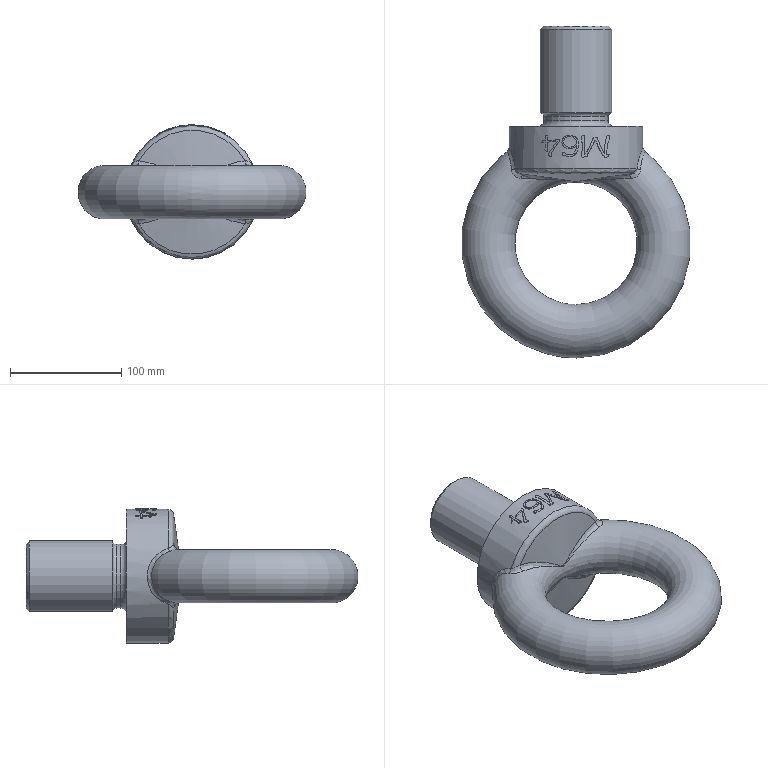Part | STEP file | solid 44 | 1 solid | 104 faces | box 206 x 298 x 120.501 mm | volume 1511005 mm3 | other 73 | plane 8 | spline 8 | cylinder 7 | torus 5 | cone 3 | commonest cylinder face diameters 121 x3 120 x2 57.8 x1 64 x1